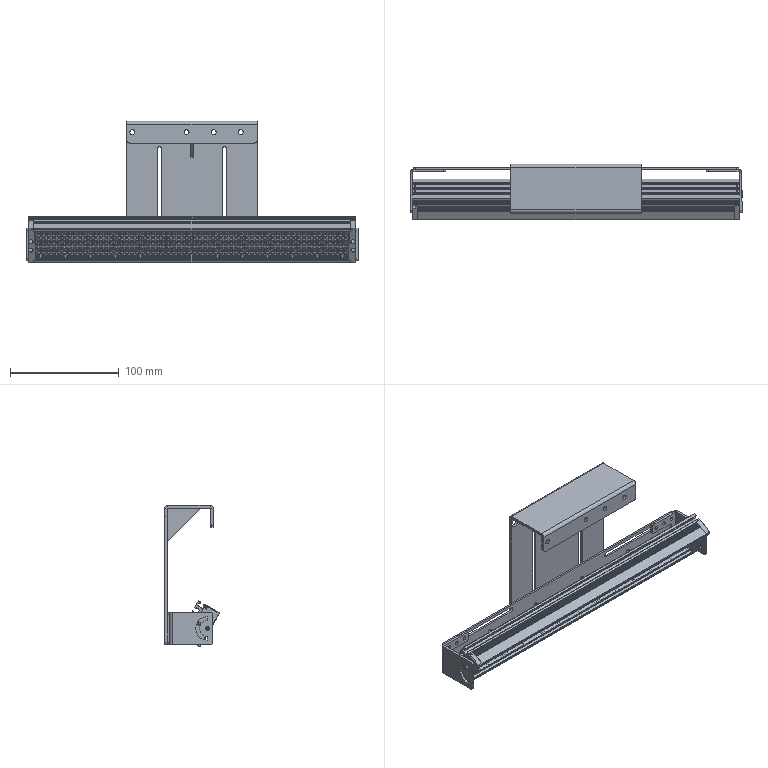Part | SolidWorks | 19 solids | 2235 faces | box 306 x 50.679 x 130.275 mm | volume 162971 mm3 | spline 720 | plane 676 | cylinder 659 | cone 180 | commonest cylinder face diameters 2 x290 1.9 x144 0.2 x66 3.3 x32 0.6 x24 4 x24